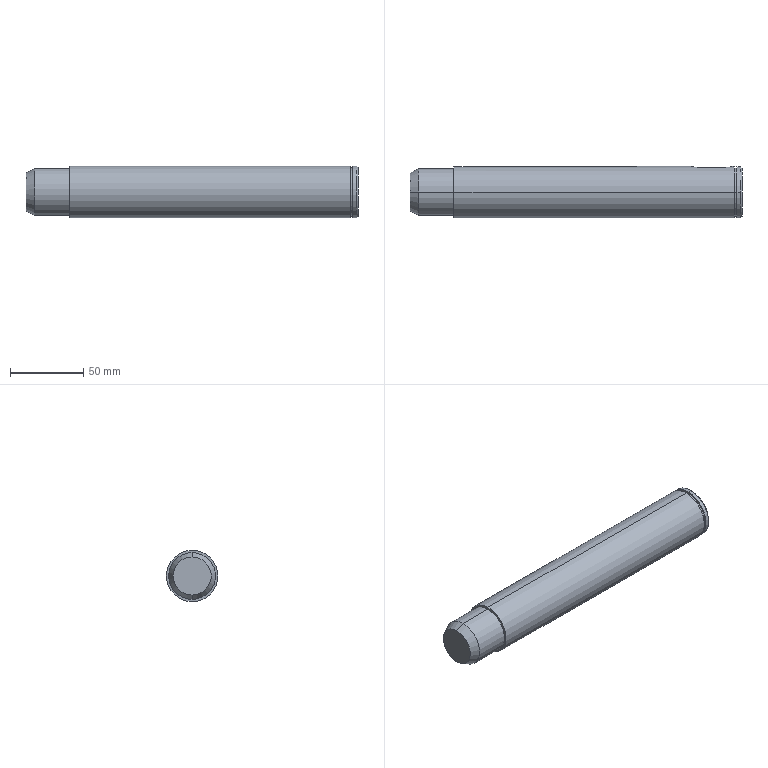Part | STEP file | 02-Support shaft 5 | 1 solid | 22 faces | box 226.5 x 35 x 35 mm | volume 210864 mm3 | cylinder 10 | plane 8 | cone 4 | commonest cylinder face diameters 35 x4 10 x2 32 x2 33 x2